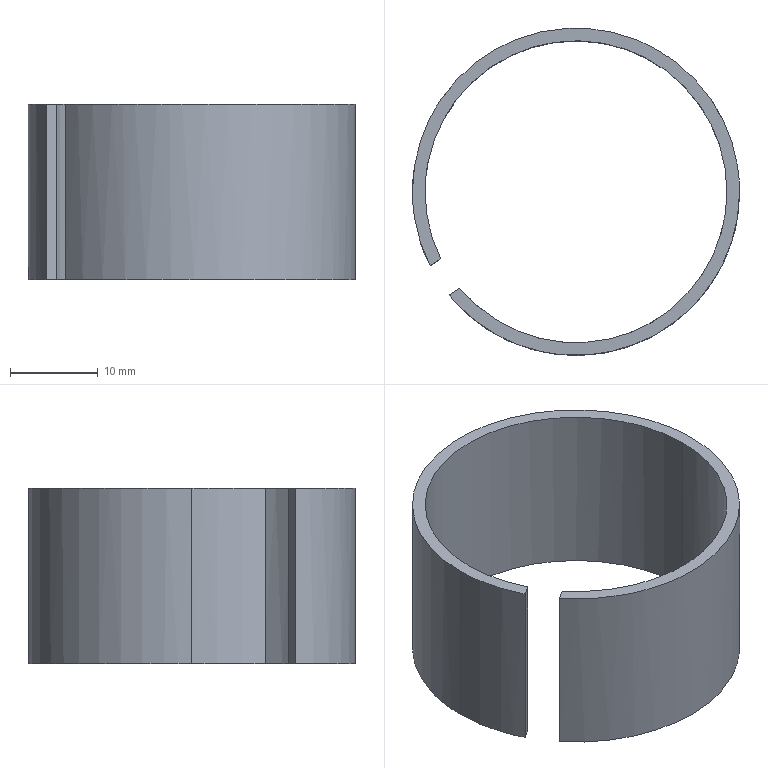Part | STEP file | Jaqueta-A | 1 solid | 10 faces | box 37.28 x 37.28 x 20 mm | volume 3130 mm3 | cylinder 6 | plane 4 | commonest cylinder face diameters 34.4 x3 37.28 x3